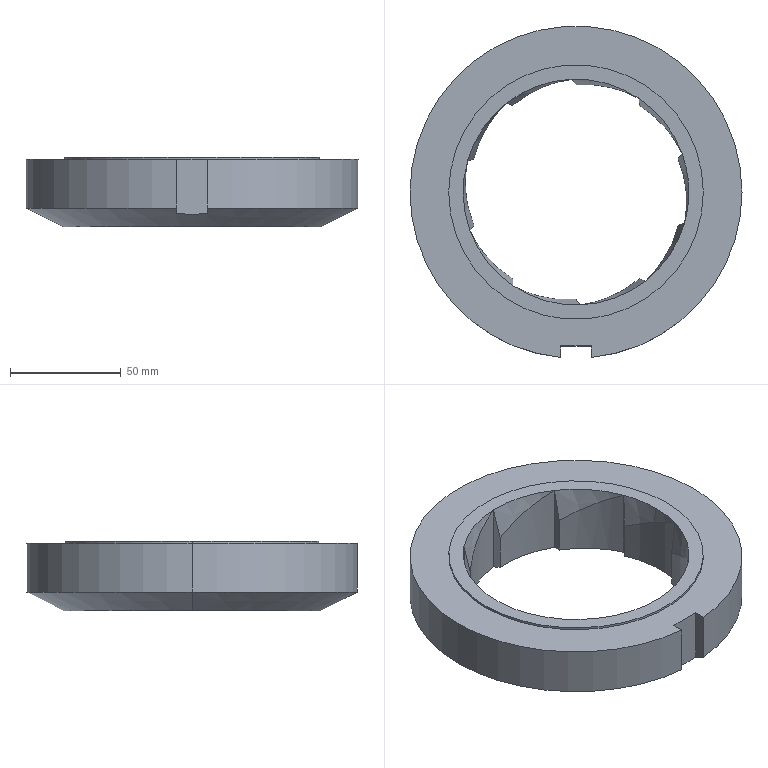Part | SolidWorks | features BaseBody 1, ICE 1 | 1 solid | 45 faces | box 150 x 149.673 x 31.5 mm | volume 269452 mm3 | cylinder 16 | plane 16 | cone 13 | commonest cylinder face diameters 100 x11 150 x3 115 x2
STEP:
#1=CARTESIAN_POINT('',(567.357,249.731,-666.693));
#2=VERTEX_POINT('',#1);
#3=CARTESIAN_POINT('',(571.036,234.744,-658.862));
#4=VERTEX_POINT('',#3);
#5=CARTESIAN_POINT('',(567.357,249.731,-666.693));
#6=CARTESIAN_POINT('',(568.37,247.306,-665.409));
#7=CARTESIAN_POINT('',(569.175,244.843,-664.114));
#8=CARTESIAN_POINT('',(570.398,239.847,-661.503));
#9=CARTESIAN_POINT('',(570.815,237.313,-660.187));
#10=CARTESIAN_POINT('',(571.036,234.744,-658.862));
#11=B_SPLINE_CURVE_WITH_KNOTS('',3,(#5,#6,#7,#8,#9,#10),.UNSPECIFIED.,.F.,.F.,(4,2,4),(0.000000238,0.008649,0.0173),.UNSPECIFIED.);
#12=EDGE_CURVE('',#2,#4,#11,.T.);
#13=ORIENTED_EDGE('',*,*,#12,.T.);
#14=CARTESIAN_POINT('',(572.231,234.744,-651.693));
#15=VERTEX_POINT('',#14);
#16=CARTESIAN_POINT('',(572.231,234.744,-651.693));
#17=DIRECTION('',(0.1644,0.,0.9864));
#18=VECTOR('',#17,1000.);
#19=LINE('',#16,#18);
#20=EDGE_CURVE('',#4,#15,#19,.T.);
#21=ORIENTED_EDGE('',*,*,#20,.T.);
#22=CARTESIAN_POINT('',(569.155,252.187,-651.693));
#23=VERTEX_POINT('',#22);
#24=CARTESIAN_POINT('',(521.231,234.744,-651.693));
#25=DIRECTION('',(0.,0.,-1.));
#26=DIRECTION('',(-1.,0.,0.));
#27=AXIS2_PLACEMENT_3D('',#24,#25,#26);
#28=CIRCLE('',#27,51.);
#29=EDGE_CURVE('',#23,#15,#28,.T.);
#30=ORIENTED_EDGE('',*,*,#29,.F.);
#31=CARTESIAN_POINT('',(569.155,252.187,-651.693));
#32=CARTESIAN_POINT('',(568.562,251.378,-656.695));
#33=CARTESIAN_POINT('',(567.963,250.56,-661.695));
#34=CARTESIAN_POINT('',(567.357,249.731,-666.693));
#35=B_SPLINE_CURVE_WITH_KNOTS('',3,(#31,#32,#33,#34),.UNSPECIFIED.,.F.,.F.,(4,4),(0.000000204,0.01531),.UNSPECIFIED.);
#36=EDGE_CURVE('',#23,#2,#35,.T.);
#37=ORIENTED_EDGE('',*,*,#36,.T.);
#38=EDGE_LOOP('',(#13,#21,#30,#37));
#39=FACE_OUTER_BOUND('',#38,.T.);
#40=CARTESIAN_POINT('',(521.231,234.744,-651.693));
#41=DIRECTION('',(0.,0.,1.));
#42=DIRECTION('',(1.,0.,0.));
#43=AXIS2_PLACEMENT_3D('',#40,#41,#42);
#44=CONICAL_SURFACE('',#43,51.,0.1651);
#45=ADVANCED_FACE('',(#39),#44,.F.);
#46=CARTESIAN_POINT('',(463.134,234.744,-683.193));
#47=VERTEX_POINT('',#46);
#48=CARTESIAN_POINT('',(579.327,234.744,-683.193));
#49=VERTEX_POINT('',#48);
#50=CARTESIAN_POINT('',(521.231,234.744,-683.193));
#51=DIRECTION('',(0.,0.,-1.));
#52=DIRECTION('',(-1.,0.,0.));
#53=AXIS2_PLACEMENT_3D('',#50,#51,#52);
#54=CIRCLE('',#53,58.097);
#55=EDGE_CURVE('',#47,#49,#54,.T.);
#56=ORIENTED_EDGE('',*,*,#55,.F.);
#57=CARTESIAN_POINT('',(446.231,234.744,-674.693));
#58=VERTEX_POINT('',#57);
#59=CARTESIAN_POINT('',(463.731,234.744,-683.493));
#60=DIRECTION('',(-0.8934,0.,0.4493));
#61=VECTOR('',#60,1000.);
#62=LINE('',#59,#61);
#63=EDGE_CURVE('',#47,#58,#62,.T.);
#64=ORIENTED_EDGE('',*,*,#63,.T.);
#65=CARTESIAN_POINT('',(596.231,234.744,-674.693));
#66=VERTEX_POINT('',#65);
#67=CARTESIAN_POINT('',(521.231,234.744,-674.693));
#68=DIRECTION('',(0.,0.,-1.));
#69=DIRECTION('',(-1.,0.,0.));
#70=AXIS2_PLACEMENT_3D('',#67,#68,#69);
#71=CIRCLE('',#70,75.);
#72=EDGE_CURVE('',#58,#66,#71,.T.);
#73=ORIENTED_EDGE('',*,*,#72,.T.);
#74=CARTESIAN_POINT('',(578.731,234.744,-683.493));
#75=DIRECTION('',(0.8934,0.,0.4493));
#76=VECTOR('',#75,1000.);
#77=LINE('',#74,#76);
#78=EDGE_CURVE('',#49,#66,#77,.T.);
#79=ORIENTED_EDGE('',*,*,#78,.F.);
#80=EDGE_LOOP('',(#56,#64,#73,#79));
#81=FACE_OUTER_BOUND('',#80,.T.);
#82=CARTESIAN_POINT('',(521.231,234.744,-683.493));
#83=DIRECTION('',(0.,0.,1.));
#84=DIRECTION('',(1.,0.,0.));
#85=AXIS2_PLACEMENT_3D('',#82,#83,#84);
#86=CONICAL_SURFACE('',#85,57.5,1.105);
#87=ADVANCED_FACE('',(#81),#86,.T.);
#88=CARTESIAN_POINT('',(578.731,234.744,-652.693));
#89=VERTEX_POINT('',#88);
#90=CARTESIAN_POINT('',(463.731,234.744,-652.693));
#91=VERTEX_POINT('',#90);
#92=CARTESIAN_POINT('',(521.231,234.744,-652.693));
#93=DIRECTION('',(0.,0.,1.));
#94=DIRECTION('',(1.,0.,0.));
#95=AXIS2_PLACEMENT_3D('',#92,#93,#94);
#96=CIRCLE('',#95,57.5);
#97=EDGE_CURVE('',#89,#91,#96,.T.);
#98=ORIENTED_EDGE('',*,*,#97,.T.);
#99=CARTESIAN_POINT('',(463.731,234.744,-651.693));
#100=VERTEX_POINT('',#99);
#101=CARTESIAN_POINT('',(463.731,234.744,-652.693));
#102=DIRECTION('',(0.,0.,1.));
#103=VECTOR('',#102,1000.);
#104=LINE('',#101,#103);
#105=EDGE_CURVE('',#91,#100,#104,.T.);
#106=ORIENTED_EDGE('',*,*,#105,.T.);
#107=CARTESIAN_POINT('',(578.731,234.744,-651.693));
#108=VERTEX_POINT('',#107);
#109=CARTESIAN_POINT('',(521.231,234.744,-651.693));
#110=DIRECTION('',(0.,0.,1.));
#111=DIRECTION('',(1.,0.,0.));
#112=AXIS2_PLACEMENT_3D('',#109,#110,#111);
#113=CIRCLE('',#112,57.5);
#114=EDGE_CURVE('',#108,#100,#113,.T.);
#115=ORIENTED_EDGE('',*,*,#114,.F.);
#116=CARTESIAN_POINT('',(578.731,234.744,-652.693));
#117=DIRECTION('',(0.,0.,1.));
#118=VECTOR('',#117,1000.);
#119=LINE('',#116,#118);
#120=EDGE_CURVE('',#89,#108,#119,.T.);
#121=ORIENTED_EDGE('',*,*,#120,.F.);
#122=EDGE_LOOP('',(#98,#106,#115,#121));
#123=FACE_OUTER_BOUND('',#122,.T.);
#124=CARTESIAN_POINT('',(521.231,234.744,-652.693));
#125=DIRECTION('',(0.,0.,1.));
#126=DIRECTION('',(1.,0.,0.));
#127=AXIS2_PLACEMENT_3D('',#124,#125,#126);
#128=CYLINDRICAL_SURFACE('',#127,57.5);
#129=ADVANCED_FACE('',(#123),#128,.T.);
#130=ORIENTED_EDGE('',*,*,#72,.F.);
#131=CARTESIAN_POINT('',(446.231,234.744,-652.693));
#132=VERTEX_POINT('',#131);
#133=CARTESIAN_POINT('',(446.231,234.744,-684.693));
#134=DIRECTION('',(0.,0.,1.));
#135=VECTOR('',#134,1000.);
#136=LINE('',#133,#135);
#137=EDGE_CURVE('',#58,#132,#136,.T.);
#138=ORIENTED_EDGE('',*,*,#137,.T.);
#139=CARTESIAN_POINT('',(596.231,234.744,-652.693));
#140=VERTEX_POINT('',#139);
#141=CARTESIAN_POINT('',(521.231,234.744,-652.693));
#142=DIRECTION('',(0.,0.,1.));
#143=DIRECTION('',(1.,0.,0.));
#144=AXIS2_PLACEMENT_3D('',#141,#142,#143);
#145=CIRCLE('',#144,75.);
#146=EDGE_CURVE('',#140,#132,#145,.T.);
#147=ORIENTED_EDGE('',*,*,#146,.F.);
#148=CARTESIAN_POINT('',(596.231,234.744,-684.693));
#149=DIRECTION('',(0.,0.,1.));
#150=VECTOR('',#149,1000.);
#151=LINE('',#148,#150);
#152=EDGE_CURVE('',#66,#140,#151,.T.);
#153=ORIENTED_EDGE('',*,*,#152,.F.);
#154=EDGE_LOOP('',(#130,#138,#147,#153));
#155=FACE_OUTER_BOUND('',#154,.T.);
#156=CARTESIAN_POINT('',(521.231,234.744,-684.693));
#157=DIRECTION('',(0.,0.,1.));
#158=DIRECTION('',(1.,0.,0.));
#159=AXIS2_PLACEMENT_3D('',#156,#157,#158);
#160=CYLINDRICAL_SURFACE('',#159,75.);
#161=ADVANCED_FACE('',(#155),#160,.T.);
#162=CARTESIAN_POINT('',(528.231,160.071,-674.693));
#163=VERTEX_POINT('',#162);
#164=CARTESIAN_POINT('',(521.231,234.744,-674.693));
#165=DIRECTION('',(0.,0.,-1.));
#166=DIRECTION('',(-1.,0.,0.));
#167=AXIS2_PLACEMENT_3D('',#164,#165,#166);
#168=CIRCLE('',#167,75.);
#169=EDGE_CURVE('',#66,#163,#168,.T.);
#170=ORIENTED_EDGE('',*,*,#169,.F.);
#171=ORIENTED_EDGE('',*,*,#152,.T.);
#172=CARTESIAN_POINT('',(528.231,160.071,-652.693));
#173=VERTEX_POINT('',#172);
#174=CARTESIAN_POINT('',(521.231,234.744,-652.693));
#175=DIRECTION('',(0.,0.,1.));
#176=DIRECTION('',(1.,0.,0.));
#177=AXIS2_PLACEMENT_3D('',#174,#175,#176);
#178=CIRCLE('',#177,75.);
#179=EDGE_CURVE('',#173,#140,#178,.T.);
#180=ORIENTED_EDGE('',*,*,#179,.F.);
#181=CARTESIAN_POINT('',(528.231,160.071,-684.693));
#182=DIRECTION('',(0.,0.,-1.));
#183=VECTOR('',#182,1000.);
#184=LINE('',#181,#183);
#185=EDGE_CURVE('',#173,#163,#184,.T.);
#186=ORIENTED_EDGE('',*,*,#185,.T.);
#187=EDGE_LOOP('',(#170,#171,#180,#186));
#188=FACE_OUTER_BOUND('',#187,.T.);
#189=CARTESIAN_POINT('',(521.231,234.744,-684.693));
#190=DIRECTION('',(0.,0.,1.));
#191=DIRECTION('',(1.,0.,0.));
#192=AXIS2_PLACEMENT_3D('',#189,#190,#191);
#193=CYLINDRICAL_SURFACE('',#192,75.);
#194=ADVANCED_FACE('',(#188),#193,.T.);
#195=CARTESIAN_POINT('',(471.242,239.027,-656.66));
#196=VERTEX_POINT('',#195);
#197=CARTESIAN_POINT('',(472.206,248.801,-651.693));
#198=VERTEX_POINT('',#197);
#199=CARTESIAN_POINT('',(471.242,239.027,-656.66));
#200=CARTESIAN_POINT('',(471.242,242.303,-654.982));
#201=CARTESIAN_POINT('',(471.56,245.561,-653.327));
#202=CARTESIAN_POINT('',(472.206,248.801,-651.693));
#203=B_SPLINE_CURVE_WITH_KNOTS('',3,(#199,#200,#201,#202),.UNSPECIFIED.,.F.,.F.,(4,4),(0.02207,0.03297),.UNSPECIFIED.);
#204=EDGE_CURVE('',#196,#198,#203,.T.);
#205=ORIENTED_EDGE('',*,*,#204,.F.);
#206=CARTESIAN_POINT('',(471.242,239.027,-683.193));
#207=VERTEX_POINT('',#206);
#208=CARTESIAN_POINT('',(471.242,239.027,-617.693));
#209=DIRECTION('',(0.,0.,-1.));
#210=VECTOR('',#209,1000.);
#211=LINE('',#208,#210);
#212=EDGE_CURVE('',#196,#207,#211,.T.);
#213=ORIENTED_EDGE('',*,*,#212,.T.);
#214=CARTESIAN_POINT('',(472.206,248.801,-683.193));
#215=VERTEX_POINT('',#214);
#216=CARTESIAN_POINT('',(521.242,239.027,-683.193));
#217=DIRECTION('',(0.,0.,1.));
#218=DIRECTION('',(-1.,0.,0.));
#219=AXIS2_PLACEMENT_3D('',#216,#217,#218);
#220=CIRCLE('',#219,50.);
#221=EDGE_CURVE('',#215,#207,#220,.T.);
#222=ORIENTED_EDGE('',*,*,#221,.F.);
#223=CARTESIAN_POINT('',(472.206,248.801,-617.693));
#224=DIRECTION('',(0.,0.,-1.));
#225=VECTOR('',#224,1000.);
#226=LINE('',#223,#225);
#227=EDGE_CURVE('',#198,#215,#226,.T.);
#228=ORIENTED_EDGE('',*,*,#227,.F.);
#229=EDGE_LOOP('',(#205,#213,#222,#228));
#230=FACE_OUTER_BOUND('',#229,.T.);
#231=CARTESIAN_POINT('',(521.242,239.027,-617.693));
#232=DIRECTION('',(0.,0.,-1.));
#233=DIRECTION('',(-1.,0.,0.));
#234=AXIS2_PLACEMENT_3D('',#231,#232,#233);
#235=CYLINDRICAL_SURFACE('',#234,50.);
#236=ADVANCED_FACE('',(#230),#235,.F.);
#237=CARTESIAN_POINT('',(521.231,186.244,-683.193));
#238=VERTEX_POINT('',#237);
#239=CARTESIAN_POINT('',(523.011,183.775,-683.193));
#240=VERTEX_POINT('',#239);
#241=CARTESIAN_POINT('',(521.231,186.244,-683.193));
#242=DIRECTION('',(0.5848,-0.8112,0.));
#243=VECTOR('',#242,1000.);
#244=LINE('',#241,#243);
#245=EDGE_CURVE('',#238,#240,#244,.T.);
#246=ORIENTED_EDGE('',*,*,#245,.F.);
#247=CARTESIAN_POINT('',(521.231,186.244,-666.693));
#248=VERTEX_POINT('',#247);
#249=CARTESIAN_POINT('',(521.231,186.244,-617.693));
#250=DIRECTION('',(0.,0.,-1.));
#251=VECTOR('',#250,1000.);
#252=LINE('',#249,#251);
#253=EDGE_CURVE('',#248,#238,#252,.T.);
#254=ORIENTED_EDGE('',*,*,#253,.F.);
#255=CARTESIAN_POINT('',(523.011,183.775,-651.693));
#256=VERTEX_POINT('',#255);
#257=CARTESIAN_POINT('',(523.011,183.775,-651.693));
#258=CARTESIAN_POINT('',(522.424,184.589,-656.695));
#259=CARTESIAN_POINT('',(521.831,185.411,-661.695));
#260=CARTESIAN_POINT('',(521.231,186.244,-666.693));
#261=B_SPLINE_CURVE_WITH_KNOTS('',3,(#257,#258,#259,#260),.UNSPECIFIED.,.F.,.F.,(4,4),(0.000000204,0.01531),.UNSPECIFIED.);
#262=EDGE_CURVE('',#256,#248,#261,.T.);
#263=ORIENTED_EDGE('',*,*,#262,.F.);
#264=CARTESIAN_POINT('',(523.011,183.775,-617.693));
#265=DIRECTION('',(0.,0.,-1.));
#266=VECTOR('',#265,1000.);
#267=LINE('',#264,#266);
#268=EDGE_CURVE('',#256,#240,#267,.T.);
#269=ORIENTED_EDGE('',*,*,#268,.T.);
#270=EDGE_LOOP('',(#246,#254,#263,#269));
#271=FACE_OUTER_BOUND('',#270,.T.);
#272=CARTESIAN_POINT('',(521.231,186.244,-617.693));
#273=DIRECTION('',(-0.8112,-0.5848,0.));
#274=DIRECTION('',(-0.5848,0.8112,0.));
#275=AXIS2_PLACEMENT_3D('',#272,#273,#274);
#276=PLANE('',#275);
#277=ADVANCED_FACE('',(#271),#276,.F.);
#278=CARTESIAN_POINT('',(492.712,192.463,-683.193));
#279=VERTEX_POINT('',#278);
#280=CARTESIAN_POINT('',(517.16,236.078,-683.193));
#281=DIRECTION('',(0.,0.,1.));
#282=DIRECTION('',(-1.,0.,0.));
#283=AXIS2_PLACEMENT_3D('',#280,#281,#282);
#284=CIRCLE('',#283,50.);
#285=EDGE_CURVE('',#279,#238,#284,.T.);
#286=ORIENTED_EDGE('',*,*,#285,.F.);
#287=CARTESIAN_POINT('',(492.712,192.463,-651.693));
#288=VERTEX_POINT('',#287);
#289=CARTESIAN_POINT('',(492.712,192.463,-617.693));
#290=DIRECTION('',(0.,0.,-1.));
#291=VECTOR('',#290,1000.);
#292=LINE('',#289,#291);
#293=EDGE_CURVE('',#288,#279,#292,.T.);
#294=ORIENTED_EDGE('',*,*,#293,.F.);
#295=CARTESIAN_POINT('',(521.231,186.244,-666.693));
#296=CARTESIAN_POINT('',(518.734,186.04,-665.47));
#297=CARTESIAN_POINT('',(516.264,186.026,-664.236));
#298=CARTESIAN_POINT('',(511.371,186.354,-661.749));
#299=CARTESIAN_POINT('',(508.948,186.696,-660.497));
#300=CARTESIAN_POINT('',(505.35,187.477,-658.605));
#301=CARTESIAN_POINT('',(504.157,187.783,-657.972));
#302=CARTESIAN_POINT('',(501.783,188.485,-656.701));
#303=CARTESIAN_POINT('',(500.608,188.881,-656.067));
#304=CARTESIAN_POINT('',(497.138,190.195,-654.176));
#305=CARTESIAN_POINT('',(494.891,191.241,-652.928));
#306=CARTESIAN_POINT('',(492.712,192.463,-651.693));
#307=B_SPLINE_CURVE_WITH_KNOTS('',3,(#295,#296,#297,#298,#299,#300,#301,#302,#303,#304,#305,#306),.UNSPECIFIED.,.F.,.F.,(4,2,2,2,2,4),(0.00000022,0.008242,0.01648,0.0206,0.02473,0.03297),.UNSPECIFIED.);
#308=EDGE_CURVE('',#248,#288,#307,.T.);
#309=ORIENTED_EDGE('',*,*,#308,.F.);
#310=ORIENTED_EDGE('',*,*,#253,.T.);
#311=EDGE_LOOP('',(#286,#294,#309,#310));
#312=FACE_OUTER_BOUND('',#311,.T.);
#313=CARTESIAN_POINT('',(517.16,236.078,-617.693));
#314=DIRECTION('',(0.,0.,-1.));
#315=DIRECTION('',(-1.,0.,0.));
#316=AXIS2_PLACEMENT_3D('',#313,#314,#315);
#317=CYLINDRICAL_SURFACE('',#316,50.);
#318=ADVANCED_FACE('',(#312),#317,.F.);
#319=CARTESIAN_POINT('',(549.738,195.507,-683.193));
#320=VERTEX_POINT('',#319);
#321=CARTESIAN_POINT('',(552.629,194.555,-683.193));
#322=VERTEX_POINT('',#321);
#323=CARTESIAN_POINT('',(549.738,195.507,-683.193));
#324=DIRECTION('',(0.9499,-0.3125,0.));
#325=VECTOR('',#324,1000.);
#326=LINE('',#323,#325);
#327=EDGE_CURVE('',#320,#322,#326,.T.);
#328=ORIENTED_EDGE('',*,*,#327,.F.);
#329=CARTESIAN_POINT('',(549.738,195.507,-666.693));
#330=VERTEX_POINT('',#329);
#331=CARTESIAN_POINT('',(549.738,195.507,-617.693));
#332=DIRECTION('',(0.,0.,-1.));
#333=VECTOR('',#332,1000.);
#334=LINE('',#331,#333);
#335=EDGE_CURVE('',#330,#320,#334,.T.);
#336=ORIENTED_EDGE('',*,*,#335,.F.);
#337=CARTESIAN_POINT('',(552.629,194.555,-651.693));
#338=VERTEX_POINT('',#337);
#339=CARTESIAN_POINT('',(552.629,194.555,-651.693));
#340=CARTESIAN_POINT('',(551.676,194.869,-656.695));
#341=CARTESIAN_POINT('',(550.714,195.186,-661.695));
#342=CARTESIAN_POINT('',(549.738,195.507,-666.693));
#343=B_SPLINE_CURVE_WITH_KNOTS('',3,(#339,#340,#341,#342),.UNSPECIFIED.,.F.,.F.,(4,4),(0.000000204,0.01531),.UNSPECIFIED.);
#344=EDGE_CURVE('',#338,#330,#343,.T.);
#345=ORIENTED_EDGE('',*,*,#344,.F.);
#346=CARTESIAN_POINT('',(552.629,194.555,-617.693));
#347=DIRECTION('',(0.,0.,-1.));
#348=VECTOR('',#347,1000.);
#349=LINE('',#346,#348);
#350=EDGE_CURVE('',#338,#322,#349,.T.);
#351=ORIENTED_EDGE('',*,*,#350,.T.);
#352=EDGE_LOOP('',(#328,#336,#345,#351));
#353=FACE_OUTER_BOUND('',#352,.T.);
#354=CARTESIAN_POINT('',(549.738,195.507,-617.693));
#355=DIRECTION('',(-0.3125,-0.9499,0.));
#356=DIRECTION('',(-0.9499,0.3125,0.));
#357=AXIS2_PLACEMENT_3D('',#354,#355,#356);
#358=PLANE('',#357);
#359=ADVANCED_FACE('',(#353),#358,.F.);
#360=CARTESIAN_POINT('',(567.357,219.757,-683.193));
#361=VERTEX_POINT('',#360);
#362=CARTESIAN_POINT('',(518.704,231.285,-683.193));
#363=DIRECTION('',(0.,0.,1.));
#364=DIRECTION('',(-1.,0.,0.));
#365=AXIS2_PLACEMENT_3D('',#362,#363,#364);
#366=CIRCLE('',#365,50.);
#367=EDGE_CURVE('',#322,#361,#366,.T.);
#368=ORIENTED_EDGE('',*,*,#367,.F.);
#369=ORIENTED_EDGE('',*,*,#350,.F.);
#370=CARTESIAN_POINT('',(567.357,219.757,-666.693));
#371=VERTEX_POINT('',#370);
#372=CARTESIAN_POINT('',(567.357,219.757,-666.693));
#373=CARTESIAN_POINT('',(566.779,217.319,-665.47));
#374=CARTESIAN_POINT('',(566.029,214.965,-664.236));
#375=CARTESIAN_POINT('',(564.205,210.413,-661.749));
#376=CARTESIAN_POINT('',(563.131,208.215,-660.497));
#377=CARTESIAN_POINT('',(561.277,205.035,-658.605));
#378=CARTESIAN_POINT('',(560.618,203.994,-657.972));
#379=CARTESIAN_POINT('',(559.216,201.954,-656.701));
#380=CARTESIAN_POINT('',(558.476,200.958,-656.067));
#381=CARTESIAN_POINT('',(556.154,198.064,-654.176));
#382=CARTESIAN_POINT('',(554.465,196.25,-652.928));
#383=CARTESIAN_POINT('',(552.629,194.555,-651.693));
#384=B_SPLINE_CURVE_WITH_KNOTS('',3,(#372,#373,#374,#375,#376,#377,#378,#379,#380,#381,#382,#383),.UNSPECIFIED.,.F.,.F.,(4,2,2,2,2,4),(0.000000225,0.008242,0.01648,0.0206,0.02473,0.03297),.UNSPECIFIED.);
#385=EDGE_CURVE('',#371,#338,#384,.T.);
#386=ORIENTED_EDGE('',*,*,#385,.F.);
#387=CARTESIAN_POINT('',(567.357,219.757,-617.693));
#388=DIRECTION('',(0.,0.,-1.));
#389=VECTOR('',#388,1000.);
#390=LINE('',#387,#389);
#391=EDGE_CURVE('',#371,#361,#390,.T.);
#392=ORIENTED_EDGE('',*,*,#391,.T.);
#393=EDGE_LOOP('',(#368,#369,#386,#392));
#394=FACE_OUTER_BOUND('',#393,.T.);
#395=CARTESIAN_POINT('',(518.704,231.285,-617.693));
#396=DIRECTION('',(0.,0.,-1.));
#397=DIRECTION('',(-1.,0.,0.));
#398=AXIS2_PLACEMENT_3D('',#395,#396,#397);
#399=CYLINDRICAL_SURFACE('',#398,50.);
#400=ADVANCED_FACE('',(#394),#399,.F.);
#401=CARTESIAN_POINT('',(570.255,220.686,-683.193));
#402=VERTEX_POINT('',#401);
#403=CARTESIAN_POINT('',(567.357,219.757,-683.193));
#404=DIRECTION('',(0.9522,0.3055,0.));
#405=VECTOR('',#404,1000.);
#406=LINE('',#403,#405);
#407=EDGE_CURVE('',#361,#402,#406,.T.);
#408=ORIENTED_EDGE('',*,*,#407,.F.);
#409=ORIENTED_EDGE('',*,*,#391,.F.);
#410=CARTESIAN_POINT('',(570.255,220.686,-651.693));
#411=VERTEX_POINT('',#410);
#412=CARTESIAN_POINT('',(570.255,220.686,-651.693));
#413=CARTESIAN_POINT('',(569.3,220.38,-656.695));
#414=CARTESIAN_POINT('',(568.335,220.07,-661.695));
#415=CARTESIAN_POINT('',(567.357,219.757,-666.693));
#416=B_SPLINE_CURVE_WITH_KNOTS('',3,(#412,#413,#414,#415),.UNSPECIFIED.,.F.,.F.,(4,4),(0.000000204,0.01531),.UNSPECIFIED.);
#417=EDGE_CURVE('',#411,#371,#416,.T.);
#418=ORIENTED_EDGE('',*,*,#417,.F.);
#419=CARTESIAN_POINT('',(570.255,220.686,-617.693));
#420=DIRECTION('',(0.,0.,-1.));
#421=VECTOR('',#420,1000.);
#422=LINE('',#419,#421);
#423=EDGE_CURVE('',#411,#402,#422,.T.);
#424=ORIENTED_EDGE('',*,*,#423,.T.);
#425=EDGE_LOOP('',(#408,#409,#418,#424));
#426=FACE_OUTER_BOUND('',#425,.T.);
#427=CARTESIAN_POINT('',(567.357,219.757,-617.693));
#428=DIRECTION('',(0.3055,-0.9522,0.));
#429=DIRECTION('',(-0.9522,-0.3055,0.));
#430=AXIS2_PLACEMENT_3D('',#427,#428,#429);
#431=PLANE('',#430);
#432=ADVANCED_FACE('',(#426),#431,.F.);
#433=CARTESIAN_POINT('',(567.357,249.731,-683.193));
#434=VERTEX_POINT('',#433);
#435=CARTESIAN_POINT('',(521.22,230.461,-683.193));
#436=DIRECTION('',(0.,0.,1.));
#437=DIRECTION('',(-1.,0.,0.));
#438=AXIS2_PLACEMENT_3D('',#435,#436,#437);
#439=CIRCLE('',#438,50.);
#440=EDGE_CURVE('',#402,#434,#439,.T.);
#441=ORIENTED_EDGE('',*,*,#440,.F.);
#442=ORIENTED_EDGE('',*,*,#423,.F.);
#443=CARTESIAN_POINT('',(571.036,234.744,-658.862));
#444=CARTESIAN_POINT('',(571.136,233.58,-658.261));
#445=CARTESIAN_POINT('',(571.196,232.409,-657.659));
#446=CARTESIAN_POINT('',(571.232,230.052,-656.45));
#447=CARTESIAN_POINT('',(571.208,228.876,-655.849));
#448=CARTESIAN_POINT('',(571.014,225.354,-654.053));
#449=CARTESIAN_POINT('',(570.719,223.016,-652.867));
#450=CARTESIAN_POINT('',(570.255,220.686,-651.693));
#451=B_SPLINE_CURVE_WITH_KNOTS('',3,(#443,#444,#445,#446,#447,#448,#449,#450),.UNSPECIFIED.,.F.,.F.,(4,2,2,4),(0.0173,0.02122,0.02513,0.03297),.UNSPECIFIED.);
#452=EDGE_CURVE('',#4,#411,#451,.T.);
#453=ORIENTED_EDGE('',*,*,#452,.F.);
#454=ORIENTED_EDGE('',*,*,#12,.F.);
#455=CARTESIAN_POINT('',(567.357,249.731,-617.693));
#456=DIRECTION('',(0.,0.,-1.));
#457=VECTOR('',#456,1000.);
#458=LINE('',#455,#457);
#459=EDGE_CURVE('',#2,#434,#458,.T.);
#460=ORIENTED_EDGE('',*,*,#459,.T.);
#461=EDGE_LOOP('',(#441,#442,#453,#454,#460));
#462=FACE_OUTER_BOUND('',#461,.T.);
#463=CARTESIAN_POINT('',(521.22,230.461,-617.693));
#464=DIRECTION('',(0.,0.,-1.));
#465=DIRECTION('',(-1.,0.,0.));
#466=AXIS2_PLACEMENT_3D('',#463,#464,#465);
#467=CYLINDRICAL_SURFACE('',#466,50.);
#468=ADVANCED_FACE('',(#462),#467,.F.);
#469=CARTESIAN_POINT('',(569.155,252.187,-683.193));
#470=VERTEX_POINT('',#469);
#471=CARTESIAN_POINT('',(567.357,249.731,-683.193));
#472=DIRECTION('',(0.5908,0.8068,0.));
#473=VECTOR('',#472,1000.);
#474=LINE('',#471,#473);
#475=EDGE_CURVE('',#434,#470,#474,.T.);
#476=ORIENTED_EDGE('',*,*,#475,.F.);
#477=ORIENTED_EDGE('',*,*,#459,.F.);
#478=ORIENTED_EDGE('',*,*,#36,.F.);
#479=CARTESIAN_POINT('',(569.155,252.187,-617.693));
#480=DIRECTION('',(0.,0.,-1.));
#481=VECTOR('',#480,1000.);
#482=LINE('',#479,#481);
#483=EDGE_CURVE('',#23,#470,#482,.T.);
#484=ORIENTED_EDGE('',*,*,#483,.T.);
#485=EDGE_LOOP('',(#476,#477,#478,#484));
#486=FACE_OUTER_BOUND('',#485,.T.);
#487=CARTESIAN_POINT('',(567.357,249.731,-617.693));
#488=DIRECTION('',(0.8068,-0.5908,0.));
#489=DIRECTION('',(-0.5908,-0.8068,0.));
#490=AXIS2_PLACEMENT_3D('',#487,#488,#489);
#491=PLANE('',#490);
#492=ADVANCED_FACE('',(#486),#491,.F.);
#493=CARTESIAN_POINT('',(549.738,273.981,-683.193));
#494=VERTEX_POINT('',#493);
#495=CARTESIAN_POINT('',(523.739,231.272,-683.193));
#496=DIRECTION('',(0.,0.,1.));
#497=DIRECTION('',(-1.,0.,0.));
#498=AXIS2_PLACEMENT_3D('',#495,#496,#497);
#499=CIRCLE('',#498,50.);
#500=EDGE_CURVE('',#470,#494,#499,.T.);
#501=ORIENTED_EDGE('',*,*,#500,.F.);
#502=ORIENTED_EDGE('',*,*,#483,.F.);
#503=CARTESIAN_POINT('',(549.738,273.981,-666.693));
#504=VERTEX_POINT('',#503);
#505=CARTESIAN_POINT('',(549.738,273.981,-666.693));
#506=CARTESIAN_POINT('',(551.878,272.679,-665.47));
#507=CARTESIAN_POINT('',(553.885,271.238,-664.236));
#508=CARTESIAN_POINT('',(557.65,268.097,-661.749));
#509=CARTESIAN_POINT('',(559.409,266.396,-660.497));
#510=CARTESIAN_POINT('',(561.861,263.649,-658.605));
#511=CARTESIAN_POINT('',(562.647,262.701,-657.972));
#512=CARTESIAN_POINT('',(564.154,260.737,-656.701));
#513=CARTESIAN_POINT('',(564.872,259.726,-656.067));
#514=CARTESIAN_POINT('',(566.907,256.624,-654.176));
#515=CARTESIAN_POINT('',(568.11,254.456,-652.928));
#516=CARTESIAN_POINT('',(569.155,252.187,-651.693));
#517=B_SPLINE_CURVE_WITH_KNOTS('',3,(#505,#506,#507,#508,#509,#510,#511,#512,#513,#514,#515,#516),.UNSPECIFIED.,.F.,.F.,(4,2,2,2,2,4),(0.000000257,0.008242,0.01648,0.0206,0.02473,0.03297),.UNSPECIFIED.);
#518=EDGE_CURVE('',#504,#23,#517,.T.);
#519=ORIENTED_EDGE('',*,*,#518,.F.);
#520=CARTESIAN_POINT('',(549.738,273.981,-617.693));
#521=DIRECTION('',(0.,0.,-1.));
#522=VECTOR('',#521,1000.);
#523=LINE('',#520,#522);
#524=EDGE_CURVE('',#504,#494,#523,.T.);
#525=ORIENTED_EDGE('',*,*,#524,.T.);
#526=EDGE_LOOP('',(#501,#502,#519,#525));
#527=FACE_OUTER_BOUND('',#526,.T.);
#528=CARTESIAN_POINT('',(523.739,231.272,-617.693));
#529=DIRECTION('',(0.,0.,-1.));
#530=DIRECTION('',(-1.,0.,0.));
#531=AXIS2_PLACEMENT_3D('',#528,#529,#530);
#532=CYLINDRICAL_SURFACE('',#531,50.);
#533=ADVANCED_FACE('',(#527),#532,.F.);
#534=CARTESIAN_POINT('',(549.749,277.025,-683.193));
#535=VERTEX_POINT('',#534);
#536=CARTESIAN_POINT('',(549.738,273.981,-683.193));
#537=DIRECTION('',(0.003697,1.,0.));
#538=VECTOR('',#537,1000.);
#539=LINE('',#536,#538);
#540=EDGE_CURVE('',#494,#535,#539,.T.);
#541=ORIENTED_EDGE('',*,*,#540,.F.);
#542=ORIENTED_EDGE('',*,*,#524,.F.);
#543=CARTESIAN_POINT('',(549.749,277.025,-651.693));
#544=VERTEX_POINT('',#543);
#545=CARTESIAN_POINT('',(549.749,277.025,-651.693));
#546=CARTESIAN_POINT('',(549.746,276.022,-656.695));
#547=CARTESIAN_POINT('',(549.742,275.008,-661.695));
#548=CARTESIAN_POINT('',(549.738,273.981,-666.693));
#549=B_SPLINE_CURVE_WITH_KNOTS('',3,(#545,#546,#547,#548),.UNSPECIFIED.,.F.,.F.,(4,4),(0.000000204,0.01531),.UNSPECIFIED.);
#550=EDGE_CURVE('',#544,#504,#549,.T.);
#551=ORIENTED_EDGE('',*,*,#550,.F.);
#552=CARTESIAN_POINT('',(549.749,277.025,-617.693));
#553=DIRECTION('',(0.,0.,-1.));
#554=VECTOR('',#553,1000.);
#555=LINE('',#552,#554);
#556=EDGE_CURVE('',#544,#535,#555,.T.);
#557=ORIENTED_EDGE('',*,*,#556,.T.);
#558=EDGE_LOOP('',(#541,#542,#551,#557));
#559=FACE_OUTER_BOUND('',#558,.T.);
#560=CARTESIAN_POINT('',(549.738,273.981,-617.693));
#561=DIRECTION('',(1.,-0.003697,0.));
#562=DIRECTION('',(-0.003697,-1.,0.));
#563=AXIS2_PLACEMENT_3D('',#560,#561,#562);
#564=PLANE('',#563);
#565=ADVANCED_FACE('',(#559),#564,.F.);
#566=CARTESIAN_POINT('',(521.231,283.244,-683.193));
#567=VERTEX_POINT('',#566);
#568=CARTESIAN_POINT('',(525.301,233.41,-683.193));
#569=DIRECTION('',(0.,0.,1.));
#570=DIRECTION('',(-1.,0.,0.));
#571=AXIS2_PLACEMENT_3D('',#568,#569,#570);
#572=CIRCLE('',#571,50.);
#573=EDGE_CURVE('',#535,#567,#572,.T.);
#574=ORIENTED_EDGE('',*,*,#573,.F.);
#575=ORIENTED_EDGE('',*,*,#556,.F.);
#576=CARTESIAN_POINT('',(521.231,283.244,-666.693));
#577=VERTEX_POINT('',#576);
#578=CARTESIAN_POINT('',(521.231,283.244,-666.693));
#579=CARTESIAN_POINT('',(523.727,283.448,-665.47));
#580=CARTESIAN_POINT('',(526.198,283.462,-664.236));
#581=CARTESIAN_POINT('',(531.091,283.134,-661.749));
#582=CARTESIAN_POINT('',(533.513,282.792,-660.497));
#583=CARTESIAN_POINT('',(537.111,282.011,-658.605));
#584=CARTESIAN_POINT('',(538.304,281.705,-657.972));
#585=CARTESIAN_POINT('',(540.678,281.003,-656.701));
#586=CARTESIAN_POINT('',(541.853,280.607,-656.067));
#587=CARTESIAN_POINT('',(545.323,279.293,-654.176));
#588=CARTESIAN_POINT('',(547.57,278.246,-652.928));
#589=CARTESIAN_POINT('',(549.749,277.025,-651.693));
#590=B_SPLINE_CURVE_WITH_KNOTS('',3,(#578,#579,#580,#581,#582,#583,#584,#585,#586,#587,#588,#589),.UNSPECIFIED.,.F.,.F.,(4,2,2,2,2,4),(0.00000022,0.008242,0.01648,0.0206,0.02473,0.03297),.UNSPECIFIED.);
#591=EDGE_CURVE('',#577,#544,#590,.T.);
#592=ORIENTED_EDGE('',*,*,#591,.F.);
#593=CARTESIAN_POINT('',(521.231,283.244,-617.693));
#594=DIRECTION('',(0.,0.,-1.));
#595=VECTOR('',#594,1000.);
#596=LINE('',#593,#595);
#597=EDGE_CURVE('',#577,#567,#596,.T.);
#598=ORIENTED_EDGE('',*,*,#597,.T.);
#599=EDGE_LOOP('',(#574,#575,#592,#598));
#600=FACE_OUTER_BOUND('',#599,.T.);
#601=CARTESIAN_POINT('',(525.301,233.41,-617.693));
#602=DIRECTION('',(0.,0.,-1.));
#603=DIRECTION('',(-1.,0.,0.));
#604=AXIS2_PLACEMENT_3D('',#601,#602,#603);
#605=CYLINDRICAL_SURFACE('',#604,50.);
#606=ADVANCED_FACE('',(#600),#605,.F.);
#607=CARTESIAN_POINT('',(519.451,285.713,-683.193));
#608=VERTEX_POINT('',#607);
#609=CARTESIAN_POINT('',(521.231,283.244,-683.193));
#610=DIRECTION('',(-0.5848,0.8112,0.));
#611=VECTOR('',#610,1000.);
#612=LINE('',#609,#611);
#613=EDGE_CURVE('',#567,#608,#612,.T.);
#614=ORIENTED_EDGE('',*,*,#613,.F.);
#615=ORIENTED_EDGE('',*,*,#597,.F.);
#616=CARTESIAN_POINT('',(519.451,285.713,-651.693));
#617=VERTEX_POINT('',#616);
#618=CARTESIAN_POINT('',(519.451,285.713,-651.693));
#619=CARTESIAN_POINT('',(520.037,284.899,-656.695));
#620=CARTESIAN_POINT('',(520.63,284.077,-661.695));
#621=CARTESIAN_POINT('',(521.231,283.244,-666.693));
#622=B_SPLINE_CURVE_WITH_KNOTS('',3,(#618,#619,#620,#621),.UNSPECIFIED.,.F.,.F.,(4,4),(0.000000204,0.01531),.UNSPECIFIED.);
#623=EDGE_CURVE('',#617,#577,#622,.T.);
#624=ORIENTED_EDGE('',*,*,#623,.F.);
#625=CARTESIAN_POINT('',(519.451,285.713,-617.693));
#626=DIRECTION('',(0.,0.,-1.));
#627=VECTOR('',#626,1000.);
#628=LINE('',#625,#627);
#629=EDGE_CURVE('',#617,#608,#628,.T.);
#630=ORIENTED_EDGE('',*,*,#629,.T.);
#631=EDGE_LOOP('',(#614,#615,#624,#630));
#632=FACE_OUTER_BOUND('',#631,.T.);
#633=CARTESIAN_POINT('',(521.231,283.244,-617.693));
#634=DIRECTION('',(0.8112,0.5848,0.));
#635=DIRECTION('',(0.5848,-0.8112,0.));
#636=AXIS2_PLACEMENT_3D('',#633,#634,#635);
#637=PLANE('',#636);
#638=ADVANCED_FACE('',(#632),#637,.F.);
#639=CARTESIAN_POINT('',(492.723,273.981,-683.193));
#640=VERTEX_POINT('',#639);
#641=CARTESIAN_POINT('',(525.308,236.057,-683.193));
#642=DIRECTION('',(0.,0.,1.));
#643=DIRECTION('',(-1.,0.,0.));
#644=AXIS2_PLACEMENT_3D('',#641,#642,#643);
#645=CIRCLE('',#644,50.);
#646=EDGE_CURVE('',#608,#640,#645,.T.);
#647=ORIENTED_EDGE('',*,*,#646,.F.);
#648=ORIENTED_EDGE('',*,*,#629,.F.);
#649=CARTESIAN_POINT('',(492.723,273.981,-666.693));
#650=VERTEX_POINT('',#649);
#651=CARTESIAN_POINT('',(492.723,273.981,-666.693));
#652=CARTESIAN_POINT('',(494.623,275.614,-665.47));
#653=CARTESIAN_POINT('',(496.613,277.077,-664.236));
#654=CARTESIAN_POINT('',(500.765,279.688,-661.749));
#655=CARTESIAN_POINT('',(502.925,280.835,-660.497));
#656=CARTESIAN_POINT('',(506.295,282.318,-658.605));
#657=CARTESIAN_POINT('',(507.44,282.772,-657.972));
#658=CARTESIAN_POINT('',(509.774,283.599,-656.701));
#659=CARTESIAN_POINT('',(510.957,283.969,-656.067));
#660=CARTESIAN_POINT('',(514.537,284.946,-654.176));
#661=CARTESIAN_POINT('',(516.97,285.42,-652.928));
#662=CARTESIAN_POINT('',(519.451,285.713,-651.693));
#663=B_SPLINE_CURVE_WITH_KNOTS('',3,(#651,#652,#653,#654,#655,#656,#657,#658,#659,#660,#661,#662),.UNSPECIFIED.,.F.,.F.,(4,2,2,2,2,4),(0.000000289,0.008242,0.01648,0.0206,0.02473,0.03297),.UNSPECIFIED.);
#664=EDGE_CURVE('',#650,#617,#663,.T.);
#665=ORIENTED_EDGE('',*,*,#664,.F.);
#666=CARTESIAN_POINT('',(492.723,273.981,-617.693));
#667=DIRECTION('',(0.,0.,-1.));
#668=VECTOR('',#667,1000.);
#669=LINE('',#666,#668);
#670=EDGE_CURVE('',#650,#640,#669,.T.);
#671=ORIENTED_EDGE('',*,*,#670,.T.);
#672=EDGE_LOOP('',(#647,#648,#665,#671));
#673=FACE_OUTER_BOUND('',#672,.T.);
#674=CARTESIAN_POINT('',(525.308,236.057,-617.693));
#675=DIRECTION('',(0.,0.,-1.));
#676=DIRECTION('',(-1.,0.,0.));
#677=AXIS2_PLACEMENT_3D('',#674,#675,#676);
#678=CYLINDRICAL_SURFACE('',#677,50.);
#679=ADVANCED_FACE('',(#673),#678,.F.);
#680=CARTESIAN_POINT('',(489.832,274.933,-683.193));
#681=VERTEX_POINT('',#680);
#682=CARTESIAN_POINT('',(492.723,273.981,-683.193));
#683=DIRECTION('',(-0.9499,0.3125,0.));
#684=VECTOR('',#683,1000.);
#685=LINE('',#682,#684);
#686=EDGE_CURVE('',#640,#681,#685,.T.);
#687=ORIENTED_EDGE('',*,*,#686,.F.);
#688=ORIENTED_EDGE('',*,*,#670,.F.);
#689=CARTESIAN_POINT('',(489.832,274.933,-651.693));
#690=VERTEX_POINT('',#689);
#691=CARTESIAN_POINT('',(489.832,274.933,-651.693));
#692=CARTESIAN_POINT('',(490.785,274.619,-656.695));
#693=CARTESIAN_POINT('',(491.748,274.302,-661.695));
#694=CARTESIAN_POINT('',(492.723,273.981,-666.693));
#695=B_SPLINE_CURVE_WITH_KNOTS('',3,(#691,#692,#693,#694),.UNSPECIFIED.,.F.,.F.,(4,4),(0.000000204,0.01531),.UNSPECIFIED.);
#696=EDGE_CURVE('',#690,#650,#695,.T.);
#697=ORIENTED_EDGE('',*,*,#696,.F.);
#698=CARTESIAN_POINT('',(489.832,274.933,-617.693));
#699=DIRECTION('',(0.,0.,-1.));
#700=VECTOR('',#699,1000.);
#701=LINE('',#698,#700);
#702=EDGE_CURVE('',#690,#681,#701,.T.);
#703=ORIENTED_EDGE('',*,*,#702,.T.);
#704=EDGE_LOOP('',(#687,#688,#697,#703));
#705=FACE_OUTER_BOUND('',#704,.T.);
#706=CARTESIAN_POINT('',(492.723,273.981,-617.693));
#707=DIRECTION('',(0.3125,0.9499,0.));
#708=DIRECTION('',(0.9499,-0.3125,0.));
#709=AXIS2_PLACEMENT_3D('',#706,#707,#708);
#710=PLANE('',#709);
#711=ADVANCED_FACE('',(#705),#710,.F.);
#712=CARTESIAN_POINT('',(475.104,249.731,-683.193));
#713=VERTEX_POINT('',#712);
#714=CARTESIAN_POINT('',(523.757,238.203,-683.193));
#715=DIRECTION('',(0.,0.,1.));
#716=DIRECTION('',(-1.,0.,0.));
#717=AXIS2_PLACEMENT_3D('',#714,#715,#716);
#718=CIRCLE('',#717,50.);
#719=EDGE_CURVE('',#681,#713,#718,.T.);
#720=ORIENTED_EDGE('',*,*,#719,.F.);
#721=ORIENTED_EDGE('',*,*,#702,.F.);
#722=CARTESIAN_POINT('',(475.104,249.731,-666.693));
#723=VERTEX_POINT('',#722);
#724=CARTESIAN_POINT('',(475.104,249.731,-666.693));
#725=CARTESIAN_POINT('',(475.682,252.169,-665.47));
#726=CARTESIAN_POINT('',(476.432,254.523,-664.236));
#727=CARTESIAN_POINT('',(478.256,259.075,-661.749));
#728=CARTESIAN_POINT('',(479.33,261.273,-660.497));
#729=CARTESIAN_POINT('',(481.185,264.453,-658.605));
#730=CARTESIAN_POINT('',(481.844,265.494,-657.972));
#731=CARTESIAN_POINT('',(483.246,267.534,-656.701));
#732=CARTESIAN_POINT('',(483.985,268.53,-656.067));
#733=CARTESIAN_POINT('',(486.307,271.423,-654.176));
#734=CARTESIAN_POINT('',(487.997,273.237,-652.928));
#735=CARTESIAN_POINT('',(489.832,274.933,-651.693));
#736=B_SPLINE_CURVE_WITH_KNOTS('',3,(#724,#725,#726,#727,#728,#729,#730,#731,#732,#733,#734,#735),.UNSPECIFIED.,.F.,.F.,(4,2,2,2,2,4),(0.000000225,0.008242,0.01648,0.0206,0.02473,0.03297),.UNSPECIFIED.);
#737=EDGE_CURVE('',#723,#690,#736,.T.);
#738=ORIENTED_EDGE('',*,*,#737,.F.);
#739=CARTESIAN_POINT('',(475.104,249.731,-617.693));
#740=DIRECTION('',(0.,0.,-1.));
#741=VECTOR('',#740,1000.);
#742=LINE('',#739,#741);
#743=EDGE_CURVE('',#723,#713,#742,.T.);
#744=ORIENTED_EDGE('',*,*,#743,.T.);
#745=EDGE_LOOP('',(#720,#721,#738,#744));
#746=FACE_OUTER_BOUND('',#745,.T.);
#747=CARTESIAN_POINT('',(523.757,238.203,-617.693));
#748=DIRECTION('',(0.,0.,-1.));
#749=DIRECTION('',(-1.,0.,0.));
#750=AXIS2_PLACEMENT_3D('',#747,#748,#749);
#751=CYLINDRICAL_SURFACE('',#750,50.);
#752=ADVANCED_FACE('',(#746),#751,.F.);
#753=CARTESIAN_POINT('',(475.104,249.731,-683.193));
#754=DIRECTION('',(-0.9522,-0.3055,0.));
#755=VECTOR('',#754,1000.);
#756=LINE('',#753,#755);
#757=EDGE_CURVE('',#713,#215,#756,.T.);
#758=ORIENTED_EDGE('',*,*,#757,.F.);
#759=ORIENTED_EDGE('',*,*,#743,.F.);
#760=CARTESIAN_POINT('',(472.206,248.801,-651.693));
#761=CARTESIAN_POINT('',(473.161,249.108,-656.695));
#762=CARTESIAN_POINT('',(474.127,249.418,-661.695));
#763=CARTESIAN_POINT('',(475.104,249.731,-666.693));
#764=B_SPLINE_CURVE_WITH_KNOTS('',3,(#760,#761,#762,#763),.UNSPECIFIED.,.F.,.F.,(4,4),(0.000000204,0.01531),.UNSPECIFIED.);
#765=EDGE_CURVE('',#198,#723,#764,.T.);
#766=ORIENTED_EDGE('',*,*,#765,.F.);
#767=ORIENTED_EDGE('',*,*,#227,.T.);
#768=EDGE_LOOP('',(#758,#759,#766,#767));
#769=FACE_OUTER_BOUND('',#768,.T.);
#770=CARTESIAN_POINT('',(475.104,249.731,-617.693));
#771=DIRECTION('',(-0.3055,0.9522,0.));
#772=DIRECTION('',(0.9522,0.3055,0.));
#773=AXIS2_PLACEMENT_3D('',#770,#771,#772);
#774=PLANE('',#773);
#775=ADVANCED_FACE('',(#769),#774,.F.);
#776=ORIENTED_EDGE('',*,*,#212,.F.);
#777=CARTESIAN_POINT('',(475.104,219.757,-666.693));
#778=VERTEX_POINT('',#777);
#779=CARTESIAN_POINT('',(475.104,219.757,-666.693));
#780=CARTESIAN_POINT('',(473.812,222.851,-665.055));
#781=CARTESIAN_POINT('',(472.856,226.006,-663.399));
#782=CARTESIAN_POINT('',(471.892,230.824,-660.89));
#783=CARTESIAN_POINT('',(471.65,232.444,-660.049));
#784=CARTESIAN_POINT('',(471.406,234.897,-658.782));
#785=CARTESIAN_POINT('',(471.344,235.718,-658.359));
#786=CARTESIAN_POINT('',(471.262,237.368,-657.511));
#787=CARTESIAN_POINT('',(471.242,238.198,-657.085));
#788=CARTESIAN_POINT('',(471.242,239.027,-656.66));
#789=B_SPLINE_CURVE_WITH_KNOTS('',3,(#779,#780,#781,#782,#783,#784,#785,#786,#787,#788),.UNSPECIFIED.,.F.,.F.,(4,2,2,2,4),(0.000000238,0.01103,0.01655,0.01931,0.02207),.UNSPECIFIED.);
#790=EDGE_CURVE('',#778,#196,#789,.T.);
#791=ORIENTED_EDGE('',*,*,#790,.F.);
#792=CARTESIAN_POINT('',(475.104,219.757,-683.193));
#793=VERTEX_POINT('',#792);
#794=CARTESIAN_POINT('',(475.104,219.757,-617.693));
#795=DIRECTION('',(0.,0.,-1.));
#796=VECTOR('',#795,1000.);
#797=LINE('',#794,#796);
#798=EDGE_CURVE('',#778,#793,#797,.T.);
#799=ORIENTED_EDGE('',*,*,#798,.T.);
#800=CARTESIAN_POINT('',(521.242,239.027,-683.193));
#801=DIRECTION('',(0.,0.,1.));
#802=DIRECTION('',(-1.,0.,0.));
#803=AXIS2_PLACEMENT_3D('',#800,#801,#802);
#804=CIRCLE('',#803,50.);
#805=EDGE_CURVE('',#207,#793,#804,.T.);
#806=ORIENTED_EDGE('',*,*,#805,.F.);
#807=EDGE_LOOP('',(#776,#791,#799,#806));
#808=FACE_OUTER_BOUND('',#807,.T.);
#809=CARTESIAN_POINT('',(521.242,239.027,-617.693));
#810=DIRECTION('',(0.,0.,-1.));
#811=DIRECTION('',(-1.,0.,0.));
#812=AXIS2_PLACEMENT_3D('',#809,#810,#811);
#813=CYLINDRICAL_SURFACE('',#812,50.);
#814=ADVANCED_FACE('',(#808),#813,.F.);
#815=CARTESIAN_POINT('',(473.306,217.301,-683.193));
#816=VERTEX_POINT('',#815);
#817=CARTESIAN_POINT('',(475.104,219.757,-683.193));
#818=DIRECTION('',(-0.5908,-0.8068,0.));
#819=VECTOR('',#818,1000.);
#820=LINE('',#817,#819);
#821=EDGE_CURVE('',#793,#816,#820,.T.);
#822=ORIENTED_EDGE('',*,*,#821,.F.);
#823=ORIENTED_EDGE('',*,*,#798,.F.);
#824=CARTESIAN_POINT('',(473.306,217.301,-651.693));
#825=VERTEX_POINT('',#824);
#826=CARTESIAN_POINT('',(473.306,217.301,-651.693));
#827=CARTESIAN_POINT('',(473.899,218.11,-656.695));
#828=CARTESIAN_POINT('',(474.498,218.928,-661.695));
#829=CARTESIAN_POINT('',(475.104,219.757,-666.693));
#830=B_SPLINE_CURVE_WITH_KNOTS('',3,(#826,#827,#828,#829),.UNSPECIFIED.,.F.,.F.,(4,4),(0.000000204,0.01531),.UNSPECIFIED.);
#831=EDGE_CURVE('',#825,#778,#830,.T.);
#832=ORIENTED_EDGE('',*,*,#831,.F.);
#833=CARTESIAN_POINT('',(473.306,217.301,-617.693));
#834=DIRECTION('',(0.,0.,-1.));
#835=VECTOR('',#834,1000.);
#836=LINE('',#833,#835);
#837=EDGE_CURVE('',#825,#816,#836,.T.);
#838=ORIENTED_EDGE('',*,*,#837,.T.);
#839=EDGE_LOOP('',(#822,#823,#832,#838));
#840=FACE_OUTER_BOUND('',#839,.T.);
#841=CARTESIAN_POINT('',(475.104,219.757,-617.693));
#842=DIRECTION('',(-0.8068,0.5908,0.));
#843=DIRECTION('',(0.5908,0.8068,0.));
#844=AXIS2_PLACEMENT_3D('',#841,#842,#843);
#845=PLANE('',#844);
#846=ADVANCED_FACE('',(#840),#845,.F.);
#847=CARTESIAN_POINT('',(492.723,195.507,-683.193));
#848=VERTEX_POINT('',#847);
#849=CARTESIAN_POINT('',(518.722,238.216,-683.193));
#850=DIRECTION('',(0.,0.,1.));
#851=DIRECTION('',(-1.,0.,0.));
#852=AXIS2_PLACEMENT_3D('',#849,#850,#851);
#853=CIRCLE('',#852,50.);
#854=EDGE_CURVE('',#816,#848,#853,.T.);
#855=ORIENTED_EDGE('',*,*,#854,.F.);
#856=ORIENTED_EDGE('',*,*,#837,.F.);
#857=CARTESIAN_POINT('',(492.723,195.507,-666.693));
#858=VERTEX_POINT('',#857);
#859=CARTESIAN_POINT('',(492.723,195.507,-666.693));
#860=CARTESIAN_POINT('',(490.584,196.809,-665.47));
#861=CARTESIAN_POINT('',(488.577,198.25,-664.236));
#862=CARTESIAN_POINT('',(484.811,201.391,-661.749));
#863=CARTESIAN_POINT('',(483.052,203.092,-660.497));
#864=CARTESIAN_POINT('',(480.601,205.839,-658.605));
#865=CARTESIAN_POINT('',(479.815,206.787,-657.972));
#866=CARTESIAN_POINT('',(478.307,208.751,-656.701));
#867=CARTESIAN_POINT('',(477.589,209.762,-656.067));
#868=CARTESIAN_POINT('',(475.554,212.864,-654.176));
#869=CARTESIAN_POINT('',(474.351,215.032,-652.928));
#870=CARTESIAN_POINT('',(473.306,217.301,-651.693));
#871=B_SPLINE_CURVE_WITH_KNOTS('',3,(#859,#860,#861,#862,#863,#864,#865,#866,#867,#868,#869,#870),.UNSPECIFIED.,.F.,.F.,(4,2,2,2,2,4),(0.000000257,0.008242,0.01648,0.0206,0.02473,0.03297),.UNSPECIFIED.);
#872=EDGE_CURVE('',#858,#825,#871,.T.);
#873=ORIENTED_EDGE('',*,*,#872,.F.);
#874=CARTESIAN_POINT('',(492.723,195.507,-617.693));
#875=DIRECTION('',(0.,0.,-1.));
#876=VECTOR('',#875,1000.);
#877=LINE('',#874,#876);
#878=EDGE_CURVE('',#858,#848,#877,.T.);
#879=ORIENTED_EDGE('',*,*,#878,.T.);
#880=EDGE_LOOP('',(#855,#856,#873,#879));
#881=FACE_OUTER_BOUND('',#880,.T.);
#882=CARTESIAN_POINT('',(518.722,238.216,-617.693));
#883=DIRECTION('',(0.,0.,-1.));
#884=DIRECTION('',(-1.,0.,0.));
#885=AXIS2_PLACEMENT_3D('',#882,#883,#884);
#886=CYLINDRICAL_SURFACE('',#885,50.);
#887=ADVANCED_FACE('',(#881),#886,.F.);
#888=CARTESIAN_POINT('',(492.723,195.507,-683.193));
#889=DIRECTION('',(-0.003697,-1.,0.));
#890=VECTOR('',#889,1000.);
#891=LINE('',#888,#890);
#892=EDGE_CURVE('',#848,#279,#891,.T.);
#893=ORIENTED_EDGE('',*,*,#892,.F.);
#894=ORIENTED_EDGE('',*,*,#878,.F.);
#895=CARTESIAN_POINT('',(492.712,192.463,-651.693));
#896=CARTESIAN_POINT('',(492.716,193.466,-656.695));
#897=CARTESIAN_POINT('',(492.719,194.48,-661.695));
#898=CARTESIAN_POINT('',(492.723,195.507,-666.693));
#899=B_SPLINE_CURVE_WITH_KNOTS('',3,(#895,#896,#897,#898),.UNSPECIFIED.,.F.,.F.,(4,4),(0.000000204,0.01531),.UNSPECIFIED.);
#900=EDGE_CURVE('',#288,#858,#899,.T.);
#901=ORIENTED_EDGE('',*,*,#900,.F.);
#902=ORIENTED_EDGE('',*,*,#293,.T.);
#903=EDGE_LOOP('',(#893,#894,#901,#902));
#904=FACE_OUTER_BOUND('',#903,.T.);
#905=CARTESIAN_POINT('',(492.723,195.507,-617.693));
#906=DIRECTION('',(-1.,0.003697,0.));
#907=DIRECTION('',(0.003697,1.,0.));
#908=AXIS2_PLACEMENT_3D('',#905,#906,#907);
#909=PLANE('',#908);
#910=ADVANCED_FACE('',(#904),#909,.F.);
#911=CARTESIAN_POINT('',(517.154,233.431,-683.193));
#912=DIRECTION('',(0.,0.,1.));
#913=DIRECTION('',(-1.,0.,0.));
#914=AXIS2_PLACEMENT_3D('',#911,#912,#913);
#915=CIRCLE('',#914,50.);
#916=EDGE_CURVE('',#240,#320,#915,.T.);
#917=ORIENTED_EDGE('',*,*,#916,.F.);
#918=ORIENTED_EDGE('',*,*,#268,.F.);
#919=CARTESIAN_POINT('',(549.738,195.507,-666.693));
#920=CARTESIAN_POINT('',(547.838,193.874,-665.47));
#921=CARTESIAN_POINT('',(545.848,192.411,-664.236));
#922=CARTESIAN_POINT('',(541.697,189.8,-661.749));
#923=CARTESIAN_POINT('',(539.536,188.653,-660.497));
#924=CARTESIAN_POINT('',(536.166,187.17,-658.605));
#925=CARTESIAN_POINT('',(535.021,186.716,-657.972));
#926=CARTESIAN_POINT('',(532.687,185.889,-656.701));
#927=CARTESIAN_POINT('',(531.504,185.518,-656.067));
#928=CARTESIAN_POINT('',(527.925,184.542,-654.176));
#929=CARTESIAN_POINT('',(525.492,184.068,-652.928));
#930=CARTESIAN_POINT('',(523.011,183.775,-651.693));
#931=B_SPLINE_CURVE_WITH_KNOTS('',3,(#919,#920,#921,#922,#923,#924,#925,#926,#927,#928,#929,#930),.UNSPECIFIED.,.F.,.F.,(4,2,2,2,2,4),(0.000000289,0.008242,0.01648,0.0206,0.02473,0.03297),.UNSPECIFIED.);
#932=EDGE_CURVE('',#330,#256,#931,.T.);
#933=ORIENTED_EDGE('',*,*,#932,.F.);
#934=ORIENTED_EDGE('',*,*,#335,.T.);
#935=EDGE_LOOP('',(#917,#918,#933,#934));
#936=FACE_OUTER_BOUND('',#935,.T.);
#937=CARTESIAN_POINT('',(517.154,233.431,-617.693));
#938=DIRECTION('',(0.,0.,-1.));
#939=DIRECTION('',(-1.,0.,0.));
#940=AXIS2_PLACEMENT_3D('',#937,#938,#939);
#941=CYLINDRICAL_SURFACE('',#940,50.);
#942=ADVANCED_FACE('',(#936),#941,.F.);
#943=ORIENTED_EDGE('',*,*,#137,.F.);
#944=CARTESIAN_POINT('',(514.231,160.071,-674.693));
#945=VERTEX_POINT('',#944);
#946=CARTESIAN_POINT('',(521.231,234.744,-674.693));
#947=DIRECTION('',(0.,0.,-1.));
#948=DIRECTION('',(-1.,0.,0.));
#949=AXIS2_PLACEMENT_3D('',#946,#947,#948);
#950=CIRCLE('',#949,75.);
#951=EDGE_CURVE('',#945,#58,#950,.T.);
#952=ORIENTED_EDGE('',*,*,#951,.F.);
#953=CARTESIAN_POINT('',(514.231,160.071,-652.693));
#954=VERTEX_POINT('',#953);
#955=CARTESIAN_POINT('',(514.231,160.071,-684.693));
#956=DIRECTION('',(0.,0.,1.));
#957=VECTOR('',#956,1000.);
#958=LINE('',#955,#957);
#959=EDGE_CURVE('',#945,#954,#958,.T.);
#960=ORIENTED_EDGE('',*,*,#959,.T.);
#961=CARTESIAN_POINT('',(521.231,234.744,-652.693));
#962=DIRECTION('',(0.,0.,1.));
#963=DIRECTION('',(1.,0.,0.));
#964=AXIS2_PLACEMENT_3D('',#961,#962,#963);
#965=CIRCLE('',#964,75.);
#966=EDGE_CURVE('',#132,#954,#965,.T.);
#967=ORIENTED_EDGE('',*,*,#966,.F.);
#968=EDGE_LOOP('',(#943,#952,#960,#967));
#969=FACE_OUTER_BOUND('',#968,.T.);
#970=CARTESIAN_POINT('',(521.231,234.744,-684.693));
#971=DIRECTION('',(0.,0.,1.));
#972=DIRECTION('',(1.,0.,0.));
#973=AXIS2_PLACEMENT_3D('',#970,#971,#972);
#974=CYLINDRICAL_SURFACE('',#973,75.);
#975=ADVANCED_FACE('',(#969),#974,.T.);
#976=CARTESIAN_POINT('',(528.231,165.244,-652.693));
#977=VERTEX_POINT('',#976);
#978=CARTESIAN_POINT('',(528.231,234.744,-652.693));
#979=DIRECTION('',(0.,1.,0.));
#980=VECTOR('',#979,1000.);
#981=LINE('',#978,#980);
#982=EDGE_CURVE('',#173,#977,#981,.T.);
#983=ORIENTED_EDGE('',*,*,#982,.F.);
#984=ORIENTED_EDGE('',*,*,#179,.T.);
#985=ORIENTED_EDGE('',*,*,#146,.T.);
#986=ORIENTED_EDGE('',*,*,#966,.T.);
#987=CARTESIAN_POINT('',(514.231,165.244,-652.693));
#988=VERTEX_POINT('',#987);
#989=CARTESIAN_POINT('',(514.231,234.744,-652.693));
#990=DIRECTION('',(0.,-1.,0.));
#991=VECTOR('',#990,1000.);
#992=LINE('',#989,#991);
#993=EDGE_CURVE('',#988,#954,#992,.T.);
#994=ORIENTED_EDGE('',*,*,#993,.F.);
#995=CARTESIAN_POINT('',(521.231,165.244,-652.693));
#996=DIRECTION('',(-1.,0.,0.));
#997=VECTOR('',#996,1000.);
#998=LINE('',#995,#997);
#999=EDGE_CURVE('',#977,#988,#998,.T.);
#1000=ORIENTED_EDGE('',*,*,#999,.F.);
#1001=EDGE_LOOP('',(#983,#984,#985,#986,#994,#1000));
#1002=FACE_OUTER_BOUND('',#1001,.T.);
#1003=ORIENTED_EDGE('',*,*,#97,.F.);
#1004=CARTESIAN_POINT('',(521.231,234.744,-652.693));
#1005=DIRECTION('',(0.,0.,1.));
#1006=DIRECTION('',(1.,0.,0.));
#1007=AXIS2_PLACEMENT_3D('',#1004,#1005,#1006);
#1008=CIRCLE('',#1007,57.5);
#1009=EDGE_CURVE('',#91,#89,#1008,.T.);
#1010=ORIENTED_EDGE('',*,*,#1009,.F.);
#1011=EDGE_LOOP('',(#1003,#1010));
#1012=FACE_BOUND('',#1011,.T.);
#1013=CARTESIAN_POINT('',(521.231,234.744,-652.693));
#1014=DIRECTION('',(0.,0.,1.));
#1015=DIRECTION('',(1.,0.,0.));
#1016=AXIS2_PLACEMENT_3D('',#1013,#1014,#1015);
#1017=PLANE('',#1016);
#1018=ADVANCED_FACE('',(#1002,#1012),#1017,.T.);
#1019=ORIENTED_EDGE('',*,*,#105,.F.);
#1020=ORIENTED_EDGE('',*,*,#1009,.T.);
#1021=ORIENTED_EDGE('',*,*,#120,.T.);
#1022=CARTESIAN_POINT('',(521.231,234.744,-651.693));
#1023=DIRECTION('',(0.,0.,1.));
#1024=DIRECTION('',(1.,0.,0.));
#1025=AXIS2_PLACEMENT_3D('',#1022,#1023,#1024);
#1026=CIRCLE('',#1025,57.5);
#1027=EDGE_CURVE('',#100,#108,#1026,.T.);
#1028=ORIENTED_EDGE('',*,*,#1027,.F.);
#1029=EDGE_LOOP('',(#1019,#1020,#1021,#1028));
#1030=FACE_OUTER_BOUND('',#1029,.T.);
#1031=CARTESIAN_POINT('',(521.231,234.744,-652.693));
#1032=DIRECTION('',(0.,0.,1.));
#1033=DIRECTION('',(1.,0.,0.));
#1034=AXIS2_PLACEMENT_3D('',#1031,#1032,#1033);
#1035=CYLINDRICAL_SURFACE('',#1034,57.5);
#1036=ADVANCED_FACE('',(#1030),#1035,.T.);
#1037=CARTESIAN_POINT('',(521.231,234.744,-651.693));
#1038=DIRECTION('',(0.,0.,-1.));
#1039=DIRECTION('',(-1.,0.,0.));
#1040=AXIS2_PLACEMENT_3D('',#1037,#1038,#1039);
#1041=CIRCLE('',#1040,51.);
#1042=EDGE_CURVE('',#288,#825,#1041,.T.);
#1043=ORIENTED_EDGE('',*,*,#1042,.T.);
#1044=CARTESIAN_POINT('',(521.231,234.744,-651.693));
#1045=DIRECTION('',(0.,0.,-1.));
#1046=DIRECTION('',(-1.,0.,0.));
#1047=AXIS2_PLACEMENT_3D('',#1044,#1045,#1046);
#1048=CIRCLE('',#1047,51.);
#1049=EDGE_CURVE('',#825,#198,#1048,.T.);
#1050=ORIENTED_EDGE('',*,*,#1049,.T.);
#1051=CARTESIAN_POINT('',(521.231,234.744,-651.693));
#1052=DIRECTION('',(0.,0.,-1.));
#1053=DIRECTION('',(-1.,0.,0.));
#1054=AXIS2_PLACEMENT_3D('',#1051,#1052,#1053);
#1055=CIRCLE('',#1054,51.);
#1056=EDGE_CURVE('',#198,#690,#1055,.T.);
#1057=ORIENTED_EDGE('',*,*,#1056,.T.);
#1058=CARTESIAN_POINT('',(521.231,234.744,-651.693));
#1059=DIRECTION('',(0.,0.,-1.));
#1060=DIRECTION('',(-1.,0.,0.));
#1061=AXIS2_PLACEMENT_3D('',#1058,#1059,#1060);
#1062=CIRCLE('',#1061,51.);
#1063=EDGE_CURVE('',#690,#617,#1062,.T.);
#1064=ORIENTED_EDGE('',*,*,#1063,.T.);
#1065=CARTESIAN_POINT('',(521.231,234.744,-651.693));
#1066=DIRECTION('',(0.,0.,-1.));
#1067=DIRECTION('',(-1.,0.,0.));
#1068=AXIS2_PLACEMENT_3D('',#1065,#1066,#1067);
#1069=CIRCLE('',#1068,51.);
#1070=EDGE_CURVE('',#617,#544,#1069,.T.);
#1071=ORIENTED_EDGE('',*,*,#1070,.T.);
#1072=CARTESIAN_POINT('',(521.231,234.744,-651.693));
#1073=DIRECTION('',(0.,0.,-1.));
#1074=DIRECTION('',(-1.,0.,0.));
#1075=AXIS2_PLACEMENT_3D('',#1072,#1073,#1074);
#1076=CIRCLE('',#1075,51.);
#1077=EDGE_CURVE('',#544,#23,#1076,.T.);
#1078=ORIENTED_EDGE('',*,*,#1077,.T.);
#1079=ORIENTED_EDGE('',*,*,#29,.T.);
#1080=CARTESIAN_POINT('',(521.231,234.744,-651.693));
#1081=DIRECTION('',(0.,0.,-1.));
#1082=DIRECTION('',(-1.,0.,0.));
#1083=AXIS2_PLACEMENT_3D('',#1080,#1081,#1082);
#1084=CIRCLE('',#1083,51.);
#1085=EDGE_CURVE('',#15,#411,#1084,.T.);
#1086=ORIENTED_EDGE('',*,*,#1085,.T.);
#1087=CARTESIAN_POINT('',(521.231,234.744,-651.693));
#1088=DIRECTION('',(0.,0.,-1.));
#1089=DIRECTION('',(-1.,0.,0.));
#1090=AXIS2_PLACEMENT_3D('',#1087,#1088,#1089);
#1091=CIRCLE('',#1090,51.);
#1092=EDGE_CURVE('',#411,#338,#1091,.T.);
#1093=ORIENTED_EDGE('',*,*,#1092,.T.);
#1094=CARTESIAN_POINT('',(521.231,234.744,-651.693));
#1095=DIRECTION('',(0.,0.,-1.));
#1096=DIRECTION('',(-1.,0.,0.));
#1097=AXIS2_PLACEMENT_3D('',#1094,#1095,#1096);
#1098=CIRCLE('',#1097,51.);
#1099=EDGE_CURVE('',#338,#256,#1098,.T.);
#1100=ORIENTED_EDGE('',*,*,#1099,.T.);
#1101=CARTESIAN_POINT('',(521.231,234.744,-651.693));
#1102=DIRECTION('',(0.,0.,-1.));
#1103=DIRECTION('',(-1.,0.,0.));
#1104=AXIS2_PLACEMENT_3D('',#1101,#1102,#1103);
#1105=CIRCLE('',#1104,51.);
#1106=EDGE_CURVE('',#256,#288,#1105,.T.);
#1107=ORIENTED_EDGE('',*,*,#1106,.T.);
#1108=EDGE_LOOP('',(#1043,#1050,#1057,#1064,#1071,#1078,#1079,#1086,#1093,#1100,#1107));
#1109=FACE_BOUND('',#1108,.T.);
#1110=ORIENTED_EDGE('',*,*,#114,.T.);
#1111=ORIENTED_EDGE('',*,*,#1027,.T.);
#1112=EDGE_LOOP('',(#1110,#1111));
#1113=FACE_OUTER_BOUND('',#1112,.T.);
#1114=CARTESIAN_POINT('',(521.231,234.744,-651.693));
#1115=DIRECTION('',(0.,0.,-1.));
#1116=DIRECTION('',(-1.,0.,0.));
#1117=AXIS2_PLACEMENT_3D('',#1114,#1115,#1116);
#1118=PLANE('',#1117);
#1119=ADVANCED_FACE('',(#1109,#1113),#1118,.F.);
#1120=ORIENTED_EDGE('',*,*,#63,.F.);
#1121=CARTESIAN_POINT('',(521.231,234.744,-683.193));
#1122=DIRECTION('',(0.,0.,-1.));
#1123=DIRECTION('',(-1.,0.,0.));
#1124=AXIS2_PLACEMENT_3D('',#1121,#1122,#1123);
#1125=CIRCLE('',#1124,58.097);
#1126=EDGE_CURVE('',#49,#47,#1125,.T.);
#1127=ORIENTED_EDGE('',*,*,#1126,.F.);
#1128=ORIENTED_EDGE('',*,*,#78,.T.);
#1129=ORIENTED_EDGE('',*,*,#169,.T.);
#1130=CARTESIAN_POINT('',(528.231,165.244,-677.282));
#1131=VERTEX_POINT('',#1130);
#1132=CARTESIAN_POINT('',(528.231,165.244,-677.282));
#1133=CARTESIAN_POINT('',(528.231,163.52,-676.419));
#1134=CARTESIAN_POINT('',(528.231,161.795,-675.556));
#1135=CARTESIAN_POINT('',(528.231,160.071,-674.693));
#1136=B_SPLINE_CURVE_WITH_KNOTS('',3,(#1132,#1133,#1134,#1135),.UNSPECIFIED.,.F.,.F.,(4,4),(0.01526,0.02104),.UNSPECIFIED.);
#1137=EDGE_CURVE('',#1131,#163,#1136,.T.);
#1138=ORIENTED_EDGE('',*,*,#1137,.F.);
#1139=CARTESIAN_POINT('',(514.231,165.244,-677.282));
#1140=VERTEX_POINT('',#1139);
#1141=CARTESIAN_POINT('',(514.231,165.244,-677.282));
#1142=CARTESIAN_POINT('',(516.556,165.244,-677.399));
#1143=CARTESIAN_POINT('',(518.885,165.244,-677.458));
#1144=CARTESIAN_POINT('',(522.385,165.244,-677.459));
#1145=CARTESIAN_POINT('',(523.553,165.244,-677.444));
#1146=CARTESIAN_POINT('',(525.891,165.244,-677.385));
#1147=CARTESIAN_POINT('',(527.062,165.244,-677.341));
#1148=CARTESIAN_POINT('',(528.231,165.244,-677.282));
#1149=B_SPLINE_CURVE_WITH_KNOTS('',3,(#1141,#1142,#1143,#1144,#1145,#1146,#1147,#1148),.UNSPECIFIED.,.F.,.F.,(4,2,2,4),(0.01995,0.02693,0.03042,0.03391),.UNSPECIFIED.);
#1150=EDGE_CURVE('',#1140,#1131,#1149,.T.);
#1151=ORIENTED_EDGE('',*,*,#1150,.F.);
#1152=CARTESIAN_POINT('',(514.231,160.071,-674.693));
#1153=CARTESIAN_POINT('',(514.231,161.795,-675.556));
#1154=CARTESIAN_POINT('',(514.231,163.52,-676.419));
#1155=CARTESIAN_POINT('',(514.231,165.244,-677.282));
#1156=B_SPLINE_CURVE_WITH_KNOTS('',3,(#1152,#1153,#1154,#1155),.UNSPECIFIED.,.F.,.F.,(4,4),(0.01822,0.024),.UNSPECIFIED.);
#1157=EDGE_CURVE('',#945,#1140,#1156,.T.);
#1158=ORIENTED_EDGE('',*,*,#1157,.F.);
#1159=ORIENTED_EDGE('',*,*,#951,.T.);
#1160=EDGE_LOOP('',(#1120,#1127,#1128,#1129,#1138,#1151,#1158,#1159));
#1161=FACE_OUTER_BOUND('',#1160,.T.);
#1162=CARTESIAN_POINT('',(521.231,234.744,-683.493));
#1163=DIRECTION('',(0.,0.,1.));
#1164=DIRECTION('',(1.,0.,0.));
#1165=AXIS2_PLACEMENT_3D('',#1162,#1163,#1164);
#1166=CONICAL_SURFACE('',#1165,57.5,1.105);
#1167=ADVANCED_FACE('',(#1161),#1166,.T.);
#1168=ORIENTED_EDGE('',*,*,#1126,.T.);
#1169=ORIENTED_EDGE('',*,*,#55,.T.);
#1170=EDGE_LOOP('',(#1168,#1169));
#1171=FACE_OUTER_BOUND('',#1170,.T.);
#1172=ORIENTED_EDGE('',*,*,#407,.T.);
#1173=ORIENTED_EDGE('',*,*,#440,.T.);
#1174=ORIENTED_EDGE('',*,*,#475,.T.);
#1175=ORIENTED_EDGE('',*,*,#500,.T.);
#1176=ORIENTED_EDGE('',*,*,#540,.T.);
#1177=ORIENTED_EDGE('',*,*,#573,.T.);
#1178=ORIENTED_EDGE('',*,*,#613,.T.);
#1179=ORIENTED_EDGE('',*,*,#646,.T.);
#1180=ORIENTED_EDGE('',*,*,#686,.T.);
#1181=ORIENTED_EDGE('',*,*,#719,.T.);
#1182=ORIENTED_EDGE('',*,*,#757,.T.);
#1183=ORIENTED_EDGE('',*,*,#221,.T.);
#1184=ORIENTED_EDGE('',*,*,#805,.T.);
#1185=ORIENTED_EDGE('',*,*,#821,.T.);
#1186=ORIENTED_EDGE('',*,*,#854,.T.);
#1187=ORIENTED_EDGE('',*,*,#892,.T.);
#1188=ORIENTED_EDGE('',*,*,#285,.T.);
#1189=ORIENTED_EDGE('',*,*,#245,.T.);
#1190=ORIENTED_EDGE('',*,*,#916,.T.);
#1191=ORIENTED_EDGE('',*,*,#327,.T.);
#1192=ORIENTED_EDGE('',*,*,#367,.T.);
#1193=EDGE_LOOP('',(#1172,#1173,#1174,#1175,#1176,#1177,#1178,#1179,#1180,#1181,#1182,#1183,#1184,#1185,#1186,#1187,#1188,#1189,#1190,#1191,#1192));
#1194=FACE_BOUND('',#1193,.T.);
#1195=CARTESIAN_POINT('',(521.231,234.744,-683.193));
#1196=DIRECTION('',(0.,0.,-1.));
#1197=DIRECTION('',(-1.,0.,0.));
#1198=AXIS2_PLACEMENT_3D('',#1195,#1196,#1197);
#1199=PLANE('',#1198);
#1200=ADVANCED_FACE('',(#1171,#1194),#1199,.T.);
#1201=ORIENTED_EDGE('',*,*,#999,.T.);
#1202=CARTESIAN_POINT('',(514.231,165.244,-751.693));
#1203=DIRECTION('',(0.,0.,1.));
#1204=VECTOR('',#1203,1000.);
#1205=LINE('',#1202,#1204);
#1206=EDGE_CURVE('',#1140,#988,#1205,.T.);
#1207=ORIENTED_EDGE('',*,*,#1206,.F.);
#1208=ORIENTED_EDGE('',*,*,#1150,.T.);
#1209=CARTESIAN_POINT('',(528.231,165.244,-751.693));
#1210=DIRECTION('',(0.,0.,1.));
#1211=VECTOR('',#1210,1000.);
#1212=LINE('',#1209,#1211);
#1213=EDGE_CURVE('',#1131,#977,#1212,.T.);
#1214=ORIENTED_EDGE('',*,*,#1213,.T.);
#1215=EDGE_LOOP('',(#1201,#1207,#1208,#1214));
#1216=FACE_OUTER_BOUND('',#1215,.T.);
#1217=CARTESIAN_POINT('',(528.231,165.244,-751.693));
#1218=DIRECTION('',(0.,1.,0.));
#1219=DIRECTION('',(0.,0.,-1.));
#1220=AXIS2_PLACEMENT_3D('',#1217,#1218,#1219);
#1221=PLANE('',#1220);
#1222=ADVANCED_FACE('',(#1216),#1221,.F.);
#1223=ORIENTED_EDGE('',*,*,#982,.T.);
#1224=ORIENTED_EDGE('',*,*,#1213,.F.);
#1225=ORIENTED_EDGE('',*,*,#1137,.T.);
#1226=ORIENTED_EDGE('',*,*,#185,.F.);
#1227=EDGE_LOOP('',(#1223,#1224,#1225,#1226));
#1228=FACE_OUTER_BOUND('',#1227,.T.);
#1229=CARTESIAN_POINT('',(528.231,149.345,-751.693));
#1230=DIRECTION('',(1.,0.,0.));
#1231=DIRECTION('',(0.,-1.,0.));
#1232=AXIS2_PLACEMENT_3D('',#1229,#1230,#1231);
#1233=PLANE('',#1232);
#1234=ADVANCED_FACE('',(#1228),#1233,.F.);
#1235=ORIENTED_EDGE('',*,*,#993,.T.);
#1236=ORIENTED_EDGE('',*,*,#959,.F.);
#1237=ORIENTED_EDGE('',*,*,#1157,.T.);
#1238=ORIENTED_EDGE('',*,*,#1206,.T.);
#1239=EDGE_LOOP('',(#1235,#1236,#1237,#1238));
#1240=FACE_OUTER_BOUND('',#1239,.T.);
#1241=CARTESIAN_POINT('',(514.231,165.244,-751.693));
#1242=DIRECTION('',(-1.,0.,0.));
#1243=DIRECTION('',(0.,1.,0.));
#1244=AXIS2_PLACEMENT_3D('',#1241,#1242,#1243);
#1245=PLANE('',#1244);
#1246=ADVANCED_FACE('',(#1240),#1245,.F.);
#1247=ORIENTED_EDGE('',*,*,#344,.T.);
#1248=ORIENTED_EDGE('',*,*,#932,.T.);
#1249=ORIENTED_EDGE('',*,*,#1099,.F.);
#1250=EDGE_LOOP('',(#1247,#1248,#1249));
#1251=FACE_OUTER_BOUND('',#1250,.T.);
#1252=CARTESIAN_POINT('',(521.231,234.744,-651.693));
#1253=DIRECTION('',(0.,0.,1.));
#1254=DIRECTION('',(1.,0.,0.));
#1255=AXIS2_PLACEMENT_3D('',#1252,#1253,#1254);
#1256=CONICAL_SURFACE('',#1255,51.,0.1651);
#1257=ADVANCED_FACE('',(#1251),#1256,.F.);
#1258=ORIENTED_EDGE('',*,*,#872,.T.);
#1259=ORIENTED_EDGE('',*,*,#1042,.F.);
#1260=ORIENTED_EDGE('',*,*,#900,.T.);
#1261=EDGE_LOOP('',(#1258,#1259,#1260));
#1262=FACE_OUTER_BOUND('',#1261,.T.);
#1263=CARTESIAN_POINT('',(521.231,234.744,-651.693));
#1264=DIRECTION('',(0.,0.,1.));
#1265=DIRECTION('',(1.,0.,0.));
#1266=AXIS2_PLACEMENT_3D('',#1263,#1264,#1265);
#1267=CONICAL_SURFACE('',#1266,51.,0.1651);
#1268=ADVANCED_FACE('',(#1262),#1267,.F.);
#1269=ORIENTED_EDGE('',*,*,#790,.T.);
#1270=ORIENTED_EDGE('',*,*,#204,.T.);
#1271=ORIENTED_EDGE('',*,*,#1049,.F.);
#1272=ORIENTED_EDGE('',*,*,#831,.T.);
#1273=EDGE_LOOP('',(#1269,#1270,#1271,#1272));
#1274=FACE_OUTER_BOUND('',#1273,.T.);
#1275=CARTESIAN_POINT('',(521.231,234.744,-651.693));
#1276=DIRECTION('',(0.,0.,1.));
#1277=DIRECTION('',(1.,0.,0.));
#1278=AXIS2_PLACEMENT_3D('',#1275,#1276,#1277);
#1279=CONICAL_SURFACE('',#1278,51.,0.1651);
#1280=ADVANCED_FACE('',(#1274),#1279,.F.);
#1281=ORIENTED_EDGE('',*,*,#737,.T.);
#1282=ORIENTED_EDGE('',*,*,#1056,.F.);
#1283=ORIENTED_EDGE('',*,*,#765,.T.);
#1284=EDGE_LOOP('',(#1281,#1282,#1283));
#1285=FACE_OUTER_BOUND('',#1284,.T.);
#1286=CARTESIAN_POINT('',(521.231,234.744,-651.693));
#1287=DIRECTION('',(0.,0.,1.));
#1288=DIRECTION('',(1.,0.,0.));
#1289=AXIS2_PLACEMENT_3D('',#1286,#1287,#1288);
#1290=CONICAL_SURFACE('',#1289,51.,0.1651);
#1291=ADVANCED_FACE('',(#1285),#1290,.F.);
#1292=ORIENTED_EDGE('',*,*,#664,.T.);
#1293=ORIENTED_EDGE('',*,*,#1063,.F.);
#1294=ORIENTED_EDGE('',*,*,#696,.T.);
#1295=EDGE_LOOP('',(#1292,#1293,#1294));
#1296=FACE_OUTER_BOUND('',#1295,.T.);
#1297=CARTESIAN_POINT('',(521.231,234.744,-651.693));
#1298=DIRECTION('',(0.,0.,1.));
#1299=DIRECTION('',(1.,0.,0.));
#1300=AXIS2_PLACEMENT_3D('',#1297,#1298,#1299);
#1301=CONICAL_SURFACE('',#1300,51.,0.1651);
#1302=ADVANCED_FACE('',(#1296),#1301,.F.);
#1303=ORIENTED_EDGE('',*,*,#591,.T.);
#1304=ORIENTED_EDGE('',*,*,#1070,.F.);
#1305=ORIENTED_EDGE('',*,*,#623,.T.);
#1306=EDGE_LOOP('',(#1303,#1304,#1305));
#1307=FACE_OUTER_BOUND('',#1306,.T.);
#1308=CARTESIAN_POINT('',(521.231,234.744,-651.693));
#1309=DIRECTION('',(0.,0.,1.));
#1310=DIRECTION('',(1.,0.,0.));
#1311=AXIS2_PLACEMENT_3D('',#1308,#1309,#1310);
#1312=CONICAL_SURFACE('',#1311,51.,0.1651);
#1313=ADVANCED_FACE('',(#1307),#1312,.F.);
#1314=ORIENTED_EDGE('',*,*,#518,.T.);
#1315=ORIENTED_EDGE('',*,*,#1077,.F.);
#1316=ORIENTED_EDGE('',*,*,#550,.T.);
#1317=EDGE_LOOP('',(#1314,#1315,#1316));
#1318=FACE_OUTER_BOUND('',#1317,.T.);
#1319=CARTESIAN_POINT('',(521.231,234.744,-651.693));
#1320=DIRECTION('',(0.,0.,1.));
#1321=DIRECTION('',(1.,0.,0.));
#1322=AXIS2_PLACEMENT_3D('',#1319,#1320,#1321);
#1323=CONICAL_SURFACE('',#1322,51.,0.1651);
#1324=ADVANCED_FACE('',(#1318),#1323,.F.);
#1325=ORIENTED_EDGE('',*,*,#20,.F.);
#1326=ORIENTED_EDGE('',*,*,#452,.T.);
#1327=ORIENTED_EDGE('',*,*,#1085,.F.);
#1328=EDGE_LOOP('',(#1325,#1326,#1327));
#1329=FACE_OUTER_BOUND('',#1328,.T.);
#1330=CARTESIAN_POINT('',(521.231,234.744,-651.693));
#1331=DIRECTION('',(0.,0.,1.));
#1332=DIRECTION('',(1.,0.,0.));
#1333=AXIS2_PLACEMENT_3D('',#1330,#1331,#1332);
#1334=CONICAL_SURFACE('',#1333,51.,0.1651);
#1335=ADVANCED_FACE('',(#1329),#1334,.F.);
#1336=ORIENTED_EDGE('',*,*,#417,.T.);
#1337=ORIENTED_EDGE('',*,*,#385,.T.);
#1338=ORIENTED_EDGE('',*,*,#1092,.F.);
#1339=EDGE_LOOP('',(#1336,#1337,#1338));
#1340=FACE_OUTER_BOUND('',#1339,.T.);
#1341=CARTESIAN_POINT('',(521.231,234.744,-651.693));
#1342=DIRECTION('',(0.,0.,1.));
#1343=DIRECTION('',(1.,0.,0.));
#1344=AXIS2_PLACEMENT_3D('',#1341,#1342,#1343);
#1345=CONICAL_SURFACE('',#1344,51.,0.1651);
#1346=ADVANCED_FACE('',(#1340),#1345,.F.);
#1347=ORIENTED_EDGE('',*,*,#308,.T.);
#1348=ORIENTED_EDGE('',*,*,#1106,.F.);
#1349=ORIENTED_EDGE('',*,*,#262,.T.);
#1350=EDGE_LOOP('',(#1347,#1348,#1349));
#1351=FACE_OUTER_BOUND('',#1350,.T.);
#1352=CARTESIAN_POINT('',(521.231,234.744,-651.693));
#1353=DIRECTION('',(0.,0.,1.));
#1354=DIRECTION('',(1.,0.,0.));
#1355=AXIS2_PLACEMENT_3D('',#1352,#1353,#1354);
#1356=CONICAL_SURFACE('',#1355,51.,0.1651);
#1357=ADVANCED_FACE('',(#1351),#1356,.F.);
#1358=CLOSED_SHELL('',(#45,#87,#129,#161,#194,#236,#277,#318,#359,#400,#432,#468,#492,#533,#565,#606,#638,#679,#711,#752,#775,#814,#846,#887,#910,#942,#975,#1018,#1036,#1119,#1167,#1200,#1222,#1234,#1246,#1257,#1268,#1280,#1291,#1302,#1313,#1324,#1335,#1346,#1357));
#1359=MANIFOLD_SOLID_BREP('',#1358);
#1360=CARTESIAN_POINT('',(0.,0.,0.));
#1361=DIRECTION('',(0.,0.,1.));
#1362=DIRECTION('',(1.,0.,0.));
#1363=AXIS2_PLACEMENT_3D('',#1360,#1361,#1362);
#1364=(LENGTH_UNIT()NAMED_UNIT(*)SI_UNIT(.MILLI.,.METRE.));
#1365=UNCERTAINTY_MEASURE_WITH_UNIT(LENGTH_MEASURE(0.00001),#1364,'','');
#1366=(NAMED_UNIT(*)PLANE_ANGLE_UNIT()SI_UNIT($,.RADIAN.));
#1367=(NAMED_UNIT(*)SI_UNIT($,.STERADIAN.)SOLID_ANGLE_UNIT());
#1368=(GEOMETRIC_REPRESENTATION_CONTEXT(3)GLOBAL_UNCERTAINTY_ASSIGNED_CONTEXT((#1365))GLOBAL_UNIT_ASSIGNED_CONTEXT((#1364,#1366,#1367))REPRESENTATION_CONTEXT('',''));
#1369=ADVANCED_BREP_SHAPE_REPRESENTATION('',(#1359,#1363),#1368);